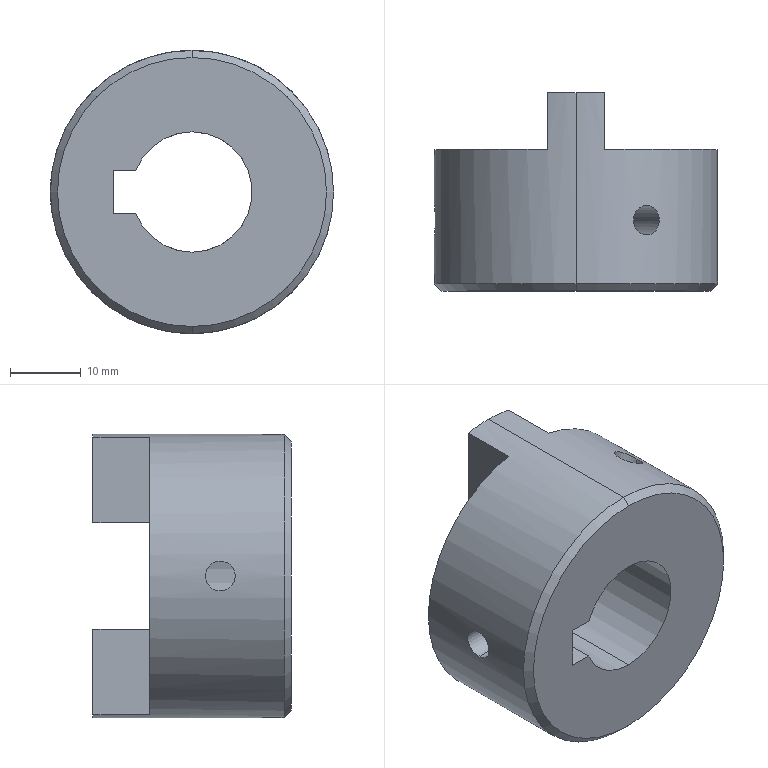Part | STEP file | CON-008 | 1 solid | 23 faces | box 40 x 28 x 40 mm | volume 21406 mm3 | plane 12 | cylinder 9 | cone 2 | commonest cylinder face diameters 4.2 x4 17 x3 40 x2